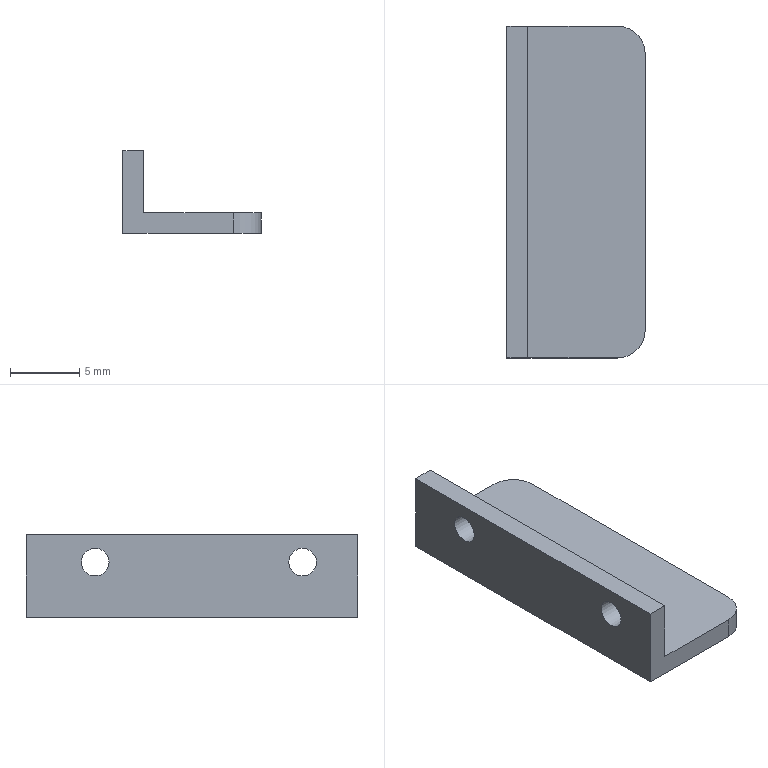Part | STEP file | 1-47.3 | 1 solid | 12 faces | box 10 x 24 x 6 mm | volume 510 mm3 | plane 8 | cylinder 4 | commonest cylinder face diameters 2 x2 4 x2
STEP:
#1=CARTESIAN_POINT('',(0.,0.,0.));
#2=DIRECTION('',(0.,0.,1.));
#3=DIRECTION('',(1.,0.,0.));
#4=AXIS2_PLACEMENT_3D('',#1,#2,#3);
#5=CARTESIAN_POINT('',(-1.5,-12.,-3.));
#6=VERTEX_POINT('',#5);
#7=CARTESIAN_POINT('',(-1.5,12.,-3.));
#8=VERTEX_POINT('',#7);
#9=CARTESIAN_POINT('',(-1.5,-12.,-3.));
#10=DIRECTION('',(0.,1.,0.));
#11=VECTOR('',#10,1.);
#12=LINE('',#9,#11);
#13=CARTESIAN_POINT('',(-1.5,0.,9.));
#14=DIRECTION('',(1.,0.,0.));
#15=DIRECTION('',(0.,1.,0.));
#16=AXIS2_PLACEMENT_3D('',#13,#14,#15);
#17=PLANE('',#16);
#18=CARTESIAN_POINT('',(-12.,-12.));
#19=DIRECTION('',(1.,0.));
#20=VECTOR('',#19,1.);
#21=LINE('',#18,#20);
#22=(GEOMETRIC_REPRESENTATION_CONTEXT(2)PARAMETRIC_REPRESENTATION_CONTEXT()REPRESENTATION_CONTEXT('',''));
#23=DEFINITIONAL_REPRESENTATION('',(#21),#22);
#24=PCURVE('',#17,#23);
#25=CARTESIAN_POINT('',(11.85,0.,-3.));
#26=DIRECTION('',(0.,0.,1.));
#27=DIRECTION('',(0.,1.,0.));
#28=AXIS2_PLACEMENT_3D('',#25,#26,#27);
#29=PLANE('',#28);
#30=CARTESIAN_POINT('',(-12.,13.35));
#31=DIRECTION('',(1.,0.));
#32=VECTOR('',#31,1.);
#33=LINE('',#30,#32);
#34=(GEOMETRIC_REPRESENTATION_CONTEXT(2)PARAMETRIC_REPRESENTATION_CONTEXT()REPRESENTATION_CONTEXT('',''));
#35=DEFINITIONAL_REPRESENTATION('',(#33),#34);
#36=PCURVE('',#29,#35);
#37=SURFACE_CURVE('',#12,(#24,#36),.PCURVE_S1.);
#38=EDGE_CURVE('',#6,#8,#37,.T.);
#39=ORIENTED_EDGE('',*,*,#38,.T.);
#40=CARTESIAN_POINT('',(-1.5,12.,3.));
#41=VERTEX_POINT('',#40);
#42=CARTESIAN_POINT('',(-1.5,12.,-3.));
#43=DIRECTION('',(0.,0.,1.));
#44=VECTOR('',#43,1.);
#45=LINE('',#42,#44);
#46=CARTESIAN_POINT('',(12.,-12.));
#47=DIRECTION('',(0.,1.));
#48=VECTOR('',#47,1.);
#49=LINE('',#46,#48);
#50=(GEOMETRIC_REPRESENTATION_CONTEXT(2)PARAMETRIC_REPRESENTATION_CONTEXT()REPRESENTATION_CONTEXT('',''));
#51=DEFINITIONAL_REPRESENTATION('',(#49),#50);
#52=PCURVE('',#17,#51);
#53=CARTESIAN_POINT('',(3.5,12.,0.));
#54=DIRECTION('',(0.,-1.,0.));
#55=DIRECTION('',(0.,0.,1.));
#56=AXIS2_PLACEMENT_3D('',#53,#54,#55);
#57=PLANE('',#56);
#58=CARTESIAN_POINT('',(-3.,5.));
#59=DIRECTION('',(1.,0.));
#60=VECTOR('',#59,1.);
#61=LINE('',#58,#60);
#62=(GEOMETRIC_REPRESENTATION_CONTEXT(2)PARAMETRIC_REPRESENTATION_CONTEXT()REPRESENTATION_CONTEXT('',''));
#63=DEFINITIONAL_REPRESENTATION('',(#61),#62);
#64=PCURVE('',#57,#63);
#65=SURFACE_CURVE('',#45,(#52,#64),.PCURVE_S1.);
#66=EDGE_CURVE('',#8,#41,#65,.T.);
#67=ORIENTED_EDGE('',*,*,#66,.T.);
#68=CARTESIAN_POINT('',(-1.5,-12.,3.));
#69=VERTEX_POINT('',#68);
#70=CARTESIAN_POINT('',(-1.5,12.,3.));
#71=DIRECTION('',(0.,-1.,0.));
#72=VECTOR('',#71,1.);
#73=LINE('',#70,#72);
#74=CARTESIAN_POINT('',(12.,-6.));
#75=DIRECTION('',(-1.,0.));
#76=VECTOR('',#75,1.);
#77=LINE('',#74,#76);
#78=(GEOMETRIC_REPRESENTATION_CONTEXT(2)PARAMETRIC_REPRESENTATION_CONTEXT()REPRESENTATION_CONTEXT('',''));
#79=DEFINITIONAL_REPRESENTATION('',(#77),#78);
#80=PCURVE('',#17,#79);
#81=CARTESIAN_POINT('',(-0.75,0.,3.));
#82=DIRECTION('',(0.,0.,-1.));
#83=DIRECTION('',(0.,-1.,0.));
#84=AXIS2_PLACEMENT_3D('',#81,#82,#83);
#85=PLANE('',#84);
#86=CARTESIAN_POINT('',(-12.,0.75));
#87=DIRECTION('',(1.,0.));
#88=VECTOR('',#87,1.);
#89=LINE('',#86,#88);
#90=(GEOMETRIC_REPRESENTATION_CONTEXT(2)PARAMETRIC_REPRESENTATION_CONTEXT()REPRESENTATION_CONTEXT('',''));
#91=DEFINITIONAL_REPRESENTATION('',(#89),#90);
#92=PCURVE('',#85,#91);
#93=SURFACE_CURVE('',#73,(#80,#92),.PCURVE_S1.);
#94=EDGE_CURVE('',#41,#69,#93,.T.);
#95=ORIENTED_EDGE('',*,*,#94,.T.);
#96=CARTESIAN_POINT('',(-1.5,-12.,3.));
#97=DIRECTION('',(0.,0.,-1.));
#98=VECTOR('',#97,1.);
#99=LINE('',#96,#98);
#100=CARTESIAN_POINT('',(-12.,-6.));
#101=DIRECTION('',(0.,-1.));
#102=VECTOR('',#101,1.);
#103=LINE('',#100,#102);
#104=(GEOMETRIC_REPRESENTATION_CONTEXT(2)PARAMETRIC_REPRESENTATION_CONTEXT()REPRESENTATION_CONTEXT('',''));
#105=DEFINITIONAL_REPRESENTATION('',(#103),#104);
#106=PCURVE('',#17,#105);
#107=CARTESIAN_POINT('',(3.5,-12.,0.));
#108=DIRECTION('',(0.,1.,0.));
#109=DIRECTION('',(0.,0.,-1.));
#110=AXIS2_PLACEMENT_3D('',#107,#108,#109);
#111=PLANE('',#110);
#112=CARTESIAN_POINT('',(-3.,5.));
#113=DIRECTION('',(1.,0.));
#114=VECTOR('',#113,1.);
#115=LINE('',#112,#114);
#116=(GEOMETRIC_REPRESENTATION_CONTEXT(2)PARAMETRIC_REPRESENTATION_CONTEXT()REPRESENTATION_CONTEXT('',''));
#117=DEFINITIONAL_REPRESENTATION('',(#115),#116);
#118=PCURVE('',#111,#117);
#119=SURFACE_CURVE('',#99,(#106,#118),.PCURVE_S1.);
#120=EDGE_CURVE('',#69,#6,#119,.T.);
#121=ORIENTED_EDGE('',*,*,#120,.T.);
#122=EDGE_LOOP('',(#39,#67,#95,#121));
#123=FACE_BOUND('',#122,.F.);
#124=CARTESIAN_POINT('',(-1.5,-7.,1.));
#125=VERTEX_POINT('',#124);
#126=CARTESIAN_POINT('',(-1.5,-8.,1.));
#127=DIRECTION('',(-1.,0.,0.));
#128=DIRECTION('',(0.,1.,0.));
#129=AXIS2_PLACEMENT_3D('',#126,#127,#128);
#130=CIRCLE('',#129,1.);
#131=CARTESIAN_POINT('',(-7.,-8.));
#132=CARTESIAN_POINT('',(-7.,-9.732));
#133=CARTESIAN_POINT('',(-8.5,-8.866));
#134=CARTESIAN_POINT('',(-10.,-8.));
#135=CARTESIAN_POINT('',(-8.5,-7.134));
#136=CARTESIAN_POINT('',(-7.,-6.268));
#137=CARTESIAN_POINT('',(-7.,-8.));
#138=(BOUNDED_CURVE()B_SPLINE_CURVE(2,(#131,#132,#133,#134,#135,#136,#137),.UNSPECIFIED.,.T.,.F.)B_SPLINE_CURVE_WITH_KNOTS((1,2,2,2,2,1),(-2.094,0.,2.094,4.189,6.283,8.378),.UNSPECIFIED.)CURVE()GEOMETRIC_REPRESENTATION_ITEM()RATIONAL_B_SPLINE_CURVE((1.,0.5,1.,0.5,1.,0.5,1.))REPRESENTATION_ITEM(''));
#139=(GEOMETRIC_REPRESENTATION_CONTEXT(2)PARAMETRIC_REPRESENTATION_CONTEXT()REPRESENTATION_CONTEXT('',''));
#140=DEFINITIONAL_REPRESENTATION('',(#138),#139);
#141=PCURVE('',#17,#140);
#142=CARTESIAN_POINT('',(0.,-8.,1.));
#143=DIRECTION('',(-1.,0.,0.));
#144=DIRECTION('',(0.,1.,0.));
#145=AXIS2_PLACEMENT_3D('',#142,#143,#144);
#146=CYLINDRICAL_SURFACE('',#145,1.);
#147=CARTESIAN_POINT('',(0.,1.5));
#148=DIRECTION('',(1.,0.));
#149=VECTOR('',#148,1.);
#150=LINE('',#147,#149);
#151=(GEOMETRIC_REPRESENTATION_CONTEXT(2)PARAMETRIC_REPRESENTATION_CONTEXT()REPRESENTATION_CONTEXT('',''));
#152=DEFINITIONAL_REPRESENTATION('',(#150),#151);
#153=PCURVE('',#146,#152);
#154=SURFACE_CURVE('',#130,(#141,#153),.PCURVE_S1.);
#155=EDGE_CURVE('',#125,#125,#154,.T.);
#156=ORIENTED_EDGE('',*,*,#155,.T.);
#157=EDGE_LOOP('',(#156));
#158=FACE_BOUND('',#157,.F.);
#159=CARTESIAN_POINT('',(-1.5,8.,1.));
#160=VERTEX_POINT('',#159);
#161=CARTESIAN_POINT('',(-1.5,7.,1.));
#162=DIRECTION('',(-1.,0.,0.));
#163=DIRECTION('',(0.,1.,0.));
#164=AXIS2_PLACEMENT_3D('',#161,#162,#163);
#165=CIRCLE('',#164,1.);
#166=CARTESIAN_POINT('',(8.,-8.));
#167=CARTESIAN_POINT('',(8.,-9.732));
#168=CARTESIAN_POINT('',(6.5,-8.866));
#169=CARTESIAN_POINT('',(5.,-8.));
#170=CARTESIAN_POINT('',(6.5,-7.134));
#171=CARTESIAN_POINT('',(8.,-6.268));
#172=CARTESIAN_POINT('',(8.,-8.));
#173=(BOUNDED_CURVE()B_SPLINE_CURVE(2,(#166,#167,#168,#169,#170,#171,#172),.UNSPECIFIED.,.T.,.F.)B_SPLINE_CURVE_WITH_KNOTS((1,2,2,2,2,1),(-2.094,0.,2.094,4.189,6.283,8.378),.UNSPECIFIED.)CURVE()GEOMETRIC_REPRESENTATION_ITEM()RATIONAL_B_SPLINE_CURVE((1.,0.5,1.,0.5,1.,0.5,1.))REPRESENTATION_ITEM(''));
#174=(GEOMETRIC_REPRESENTATION_CONTEXT(2)PARAMETRIC_REPRESENTATION_CONTEXT()REPRESENTATION_CONTEXT('',''));
#175=DEFINITIONAL_REPRESENTATION('',(#173),#174);
#176=PCURVE('',#17,#175);
#177=CARTESIAN_POINT('',(0.,7.,1.));
#178=DIRECTION('',(-1.,0.,0.));
#179=DIRECTION('',(0.,1.,0.));
#180=AXIS2_PLACEMENT_3D('',#177,#178,#179);
#181=CYLINDRICAL_SURFACE('',#180,1.);
#182=CARTESIAN_POINT('',(0.,1.5));
#183=DIRECTION('',(1.,0.));
#184=VECTOR('',#183,1.);
#185=LINE('',#182,#184);
#186=(GEOMETRIC_REPRESENTATION_CONTEXT(2)PARAMETRIC_REPRESENTATION_CONTEXT()REPRESENTATION_CONTEXT('',''));
#187=DEFINITIONAL_REPRESENTATION('',(#185),#186);
#188=PCURVE('',#181,#187);
#189=SURFACE_CURVE('',#165,(#176,#188),.PCURVE_S1.);
#190=EDGE_CURVE('',#160,#160,#189,.T.);
#191=ORIENTED_EDGE('',*,*,#190,.T.);
#192=EDGE_LOOP('',(#191));
#193=FACE_BOUND('',#192,.F.);
#194=ADVANCED_FACE('',(#123,#158,#193),#17,.F.);
#195=CARTESIAN_POINT('',(0.,12.,3.));
#196=VERTEX_POINT('',#195);
#197=CARTESIAN_POINT('',(0.,-12.,3.));
#198=VERTEX_POINT('',#197);
#199=CARTESIAN_POINT('',(0.,12.,3.));
#200=DIRECTION('',(0.,-1.,0.));
#201=VECTOR('',#200,1.);
#202=LINE('',#199,#201);
#203=CARTESIAN_POINT('',(-12.,-0.75));
#204=DIRECTION('',(1.,0.));
#205=VECTOR('',#204,1.);
#206=LINE('',#203,#205);
#207=(GEOMETRIC_REPRESENTATION_CONTEXT(2)PARAMETRIC_REPRESENTATION_CONTEXT()REPRESENTATION_CONTEXT('',''));
#208=DEFINITIONAL_REPRESENTATION('',(#206),#207);
#209=PCURVE('',#85,#208);
#210=CARTESIAN_POINT('',(0.,0.,9.));
#211=DIRECTION('',(1.,0.,0.));
#212=DIRECTION('',(0.,1.,0.));
#213=AXIS2_PLACEMENT_3D('',#210,#211,#212);
#214=PLANE('',#213);
#215=CARTESIAN_POINT('',(12.,-6.));
#216=DIRECTION('',(-1.,0.));
#217=VECTOR('',#216,1.);
#218=LINE('',#215,#217);
#219=(GEOMETRIC_REPRESENTATION_CONTEXT(2)PARAMETRIC_REPRESENTATION_CONTEXT()REPRESENTATION_CONTEXT('',''));
#220=DEFINITIONAL_REPRESENTATION('',(#218),#219);
#221=PCURVE('',#214,#220);
#222=SURFACE_CURVE('',#202,(#209,#221),.PCURVE_S1.);
#223=EDGE_CURVE('',#196,#198,#222,.T.);
#224=ORIENTED_EDGE('',*,*,#223,.T.);
#225=CARTESIAN_POINT('',(0.,-12.,3.));
#226=DIRECTION('',(-1.,0.,0.));
#227=VECTOR('',#226,1.);
#228=LINE('',#225,#227);
#229=CARTESIAN_POINT('',(12.,-0.75));
#230=DIRECTION('',(0.,1.));
#231=VECTOR('',#230,1.);
#232=LINE('',#229,#231);
#233=(GEOMETRIC_REPRESENTATION_CONTEXT(2)PARAMETRIC_REPRESENTATION_CONTEXT()REPRESENTATION_CONTEXT('',''));
#234=DEFINITIONAL_REPRESENTATION('',(#232),#233);
#235=PCURVE('',#85,#234);
#236=CARTESIAN_POINT('',(-3.,3.5));
#237=DIRECTION('',(0.,1.));
#238=VECTOR('',#237,1.);
#239=LINE('',#236,#238);
#240=(GEOMETRIC_REPRESENTATION_CONTEXT(2)PARAMETRIC_REPRESENTATION_CONTEXT()REPRESENTATION_CONTEXT('',''));
#241=DEFINITIONAL_REPRESENTATION('',(#239),#240);
#242=PCURVE('',#111,#241);
#243=SURFACE_CURVE('',#228,(#235,#242),.PCURVE_S1.);
#244=EDGE_CURVE('',#198,#69,#243,.T.);
#245=ORIENTED_EDGE('',*,*,#244,.T.);
#246=ORIENTED_EDGE('',*,*,#94,.F.);
#247=CARTESIAN_POINT('',(0.,12.,3.));
#248=DIRECTION('',(-1.,0.,0.));
#249=VECTOR('',#248,1.);
#250=LINE('',#247,#249);
#251=CARTESIAN_POINT('',(-12.,-0.75));
#252=DIRECTION('',(0.,1.));
#253=VECTOR('',#252,1.);
#254=LINE('',#251,#253);
#255=(GEOMETRIC_REPRESENTATION_CONTEXT(2)PARAMETRIC_REPRESENTATION_CONTEXT()REPRESENTATION_CONTEXT('',''));
#256=DEFINITIONAL_REPRESENTATION('',(#254),#255);
#257=PCURVE('',#85,#256);
#258=CARTESIAN_POINT('',(3.,3.5));
#259=DIRECTION('',(0.,1.));
#260=VECTOR('',#259,1.);
#261=LINE('',#258,#260);
#262=(GEOMETRIC_REPRESENTATION_CONTEXT(2)PARAMETRIC_REPRESENTATION_CONTEXT()REPRESENTATION_CONTEXT('',''));
#263=DEFINITIONAL_REPRESENTATION('',(#261),#262);
#264=PCURVE('',#57,#263);
#265=SURFACE_CURVE('',#250,(#257,#264),.PCURVE_S1.);
#266=EDGE_CURVE('',#196,#41,#265,.T.);
#267=ORIENTED_EDGE('',*,*,#266,.F.);
#268=EDGE_LOOP('',(#224,#245,#246,#267));
#269=FACE_BOUND('',#268,.F.);
#270=ADVANCED_FACE('',(#269),#85,.F.);
#271=CARTESIAN_POINT('',(0.,-7.,1.));
#272=VERTEX_POINT('',#271);
#273=CARTESIAN_POINT('',(0.,-8.,1.));
#274=DIRECTION('',(-1.,0.,0.));
#275=DIRECTION('',(0.,1.,0.));
#276=AXIS2_PLACEMENT_3D('',#273,#274,#275);
#277=CIRCLE('',#276,1.);
#278=CARTESIAN_POINT('',(0.,0.));
#279=DIRECTION('',(1.,0.));
#280=VECTOR('',#279,1.);
#281=LINE('',#278,#280);
#282=(GEOMETRIC_REPRESENTATION_CONTEXT(2)PARAMETRIC_REPRESENTATION_CONTEXT()REPRESENTATION_CONTEXT('',''));
#283=DEFINITIONAL_REPRESENTATION('',(#281),#282);
#284=PCURVE('',#146,#283);
#285=CARTESIAN_POINT('',(-7.,-8.));
#286=CARTESIAN_POINT('',(-7.,-9.732));
#287=CARTESIAN_POINT('',(-8.5,-8.866));
#288=CARTESIAN_POINT('',(-10.,-8.));
#289=CARTESIAN_POINT('',(-8.5,-7.134));
#290=CARTESIAN_POINT('',(-7.,-6.268));
#291=CARTESIAN_POINT('',(-7.,-8.));
#292=(BOUNDED_CURVE()B_SPLINE_CURVE(2,(#285,#286,#287,#288,#289,#290,#291),.UNSPECIFIED.,.T.,.F.)B_SPLINE_CURVE_WITH_KNOTS((1,2,2,2,2,1),(-2.094,0.,2.094,4.189,6.283,8.378),.UNSPECIFIED.)CURVE()GEOMETRIC_REPRESENTATION_ITEM()RATIONAL_B_SPLINE_CURVE((1.,0.5,1.,0.5,1.,0.5,1.))REPRESENTATION_ITEM(''));
#293=(GEOMETRIC_REPRESENTATION_CONTEXT(2)PARAMETRIC_REPRESENTATION_CONTEXT()REPRESENTATION_CONTEXT('',''));
#294=DEFINITIONAL_REPRESENTATION('',(#292),#293);
#295=PCURVE('',#214,#294);
#296=SURFACE_CURVE('',#277,(#284,#295),.PCURVE_S1.);
#297=EDGE_CURVE('',#272,#272,#296,.T.);
#298=ORIENTED_EDGE('',*,*,#297,.T.);
#299=CARTESIAN_POINT('',(0.,-7.,1.));
#300=DIRECTION('',(-1.,0.,0.));
#301=VECTOR('',#300,1.);
#302=LINE('',#299,#301);
#303=CARTESIAN_POINT('',(6.283,0.));
#304=DIRECTION('',(0.,1.));
#305=VECTOR('',#304,1.);
#306=LINE('',#303,#305);
#307=(GEOMETRIC_REPRESENTATION_CONTEXT(2)PARAMETRIC_REPRESENTATION_CONTEXT()REPRESENTATION_CONTEXT('',''));
#308=DEFINITIONAL_REPRESENTATION('',(#306),#307);
#309=PCURVE('',#146,#308);
#310=CARTESIAN_POINT('',(0.,0.));
#311=DIRECTION('',(0.,1.));
#312=VECTOR('',#311,1.);
#313=LINE('',#310,#312);
#314=(GEOMETRIC_REPRESENTATION_CONTEXT(2)PARAMETRIC_REPRESENTATION_CONTEXT()REPRESENTATION_CONTEXT('',''));
#315=DEFINITIONAL_REPRESENTATION('',(#313),#314);
#316=PCURVE('',#146,#315);
#317=SEAM_CURVE('',#302,(#309,#316),.PCURVE_S1.);
#318=EDGE_CURVE('',#272,#125,#317,.T.);
#319=ORIENTED_EDGE('',*,*,#318,.T.);
#320=ORIENTED_EDGE('',*,*,#155,.F.);
#321=ORIENTED_EDGE('',*,*,#318,.F.);
#322=EDGE_LOOP('',(#298,#319,#320,#321));
#323=FACE_BOUND('',#322,.F.);
#324=ADVANCED_FACE('',(#323),#146,.F.);
#325=CARTESIAN_POINT('',(0.,8.,1.));
#326=VERTEX_POINT('',#325);
#327=CARTESIAN_POINT('',(0.,7.,1.));
#328=DIRECTION('',(-1.,0.,0.));
#329=DIRECTION('',(0.,1.,0.));
#330=AXIS2_PLACEMENT_3D('',#327,#328,#329);
#331=CIRCLE('',#330,1.);
#332=CARTESIAN_POINT('',(0.,0.));
#333=DIRECTION('',(1.,0.));
#334=VECTOR('',#333,1.);
#335=LINE('',#332,#334);
#336=(GEOMETRIC_REPRESENTATION_CONTEXT(2)PARAMETRIC_REPRESENTATION_CONTEXT()REPRESENTATION_CONTEXT('',''));
#337=DEFINITIONAL_REPRESENTATION('',(#335),#336);
#338=PCURVE('',#181,#337);
#339=CARTESIAN_POINT('',(8.,-8.));
#340=CARTESIAN_POINT('',(8.,-9.732));
#341=CARTESIAN_POINT('',(6.5,-8.866));
#342=CARTESIAN_POINT('',(5.,-8.));
#343=CARTESIAN_POINT('',(6.5,-7.134));
#344=CARTESIAN_POINT('',(8.,-6.268));
#345=CARTESIAN_POINT('',(8.,-8.));
#346=(BOUNDED_CURVE()B_SPLINE_CURVE(2,(#339,#340,#341,#342,#343,#344,#345),.UNSPECIFIED.,.T.,.F.)B_SPLINE_CURVE_WITH_KNOTS((1,2,2,2,2,1),(-2.094,0.,2.094,4.189,6.283,8.378),.UNSPECIFIED.)CURVE()GEOMETRIC_REPRESENTATION_ITEM()RATIONAL_B_SPLINE_CURVE((1.,0.5,1.,0.5,1.,0.5,1.))REPRESENTATION_ITEM(''));
#347=(GEOMETRIC_REPRESENTATION_CONTEXT(2)PARAMETRIC_REPRESENTATION_CONTEXT()REPRESENTATION_CONTEXT('',''));
#348=DEFINITIONAL_REPRESENTATION('',(#346),#347);
#349=PCURVE('',#214,#348);
#350=SURFACE_CURVE('',#331,(#338,#349),.PCURVE_S1.);
#351=EDGE_CURVE('',#326,#326,#350,.T.);
#352=ORIENTED_EDGE('',*,*,#351,.T.);
#353=CARTESIAN_POINT('',(0.,8.,1.));
#354=DIRECTION('',(-1.,0.,0.));
#355=VECTOR('',#354,1.);
#356=LINE('',#353,#355);
#357=CARTESIAN_POINT('',(6.283,0.));
#358=DIRECTION('',(0.,1.));
#359=VECTOR('',#358,1.);
#360=LINE('',#357,#359);
#361=(GEOMETRIC_REPRESENTATION_CONTEXT(2)PARAMETRIC_REPRESENTATION_CONTEXT()REPRESENTATION_CONTEXT('',''));
#362=DEFINITIONAL_REPRESENTATION('',(#360),#361);
#363=PCURVE('',#181,#362);
#364=CARTESIAN_POINT('',(0.,0.));
#365=DIRECTION('',(0.,1.));
#366=VECTOR('',#365,1.);
#367=LINE('',#364,#366);
#368=(GEOMETRIC_REPRESENTATION_CONTEXT(2)PARAMETRIC_REPRESENTATION_CONTEXT()REPRESENTATION_CONTEXT('',''));
#369=DEFINITIONAL_REPRESENTATION('',(#367),#368);
#370=PCURVE('',#181,#369);
#371=SEAM_CURVE('',#356,(#363,#370),.PCURVE_S1.);
#372=EDGE_CURVE('',#326,#160,#371,.T.);
#373=ORIENTED_EDGE('',*,*,#372,.T.);
#374=ORIENTED_EDGE('',*,*,#190,.F.);
#375=ORIENTED_EDGE('',*,*,#372,.F.);
#376=EDGE_LOOP('',(#352,#373,#374,#375));
#377=FACE_BOUND('',#376,.F.);
#378=ADVANCED_FACE('',(#377),#181,.F.);
#379=ORIENTED_EDGE('',*,*,#223,.T.);
#380=CARTESIAN_POINT('',(0.,-12.,-1.5));
#381=VERTEX_POINT('',#380);
#382=CARTESIAN_POINT('',(0.,-12.,3.));
#383=DIRECTION('',(0.,0.,-1.));
#384=VECTOR('',#383,1.);
#385=LINE('',#382,#384);
#386=CARTESIAN_POINT('',(-12.,-6.));
#387=DIRECTION('',(0.,-1.));
#388=VECTOR('',#387,1.);
#389=LINE('',#386,#388);
#390=(GEOMETRIC_REPRESENTATION_CONTEXT(2)PARAMETRIC_REPRESENTATION_CONTEXT()REPRESENTATION_CONTEXT('',''));
#391=DEFINITIONAL_REPRESENTATION('',(#389),#390);
#392=PCURVE('',#214,#391);
#393=CARTESIAN_POINT('',(-3.,3.5));
#394=DIRECTION('',(1.,0.));
#395=VECTOR('',#394,1.);
#396=LINE('',#393,#395);
#397=(GEOMETRIC_REPRESENTATION_CONTEXT(2)PARAMETRIC_REPRESENTATION_CONTEXT()REPRESENTATION_CONTEXT('',''));
#398=DEFINITIONAL_REPRESENTATION('',(#396),#397);
#399=PCURVE('',#111,#398);
#400=SURFACE_CURVE('',#385,(#392,#399),.PCURVE_S1.);
#401=EDGE_CURVE('',#198,#381,#400,.T.);
#402=ORIENTED_EDGE('',*,*,#401,.T.);
#403=CARTESIAN_POINT('',(0.,12.,-1.5));
#404=VERTEX_POINT('',#403);
#405=CARTESIAN_POINT('',(0.,-12.,-1.5));
#406=DIRECTION('',(0.,1.,0.));
#407=VECTOR('',#406,1.);
#408=LINE('',#405,#407);
#409=CARTESIAN_POINT('',(-12.,-10.5));
#410=DIRECTION('',(1.,0.));
#411=VECTOR('',#410,1.);
#412=LINE('',#409,#411);
#413=(GEOMETRIC_REPRESENTATION_CONTEXT(2)PARAMETRIC_REPRESENTATION_CONTEXT()REPRESENTATION_CONTEXT('',''));
#414=DEFINITIONAL_REPRESENTATION('',(#412),#413);
#415=PCURVE('',#214,#414);
#416=CARTESIAN_POINT('',(12.,-1.682,-1.5));
#417=DIRECTION('',(0.,0.,-1.));
#418=DIRECTION('',(0.,1.,0.));
#419=AXIS2_PLACEMENT_3D('',#416,#417,#418);
#420=PLANE('',#419);
#421=CARTESIAN_POINT('',(-10.318,-12.));
#422=DIRECTION('',(1.,0.));
#423=VECTOR('',#422,1.);
#424=LINE('',#421,#423);
#425=(GEOMETRIC_REPRESENTATION_CONTEXT(2)PARAMETRIC_REPRESENTATION_CONTEXT()REPRESENTATION_CONTEXT('',''));
#426=DEFINITIONAL_REPRESENTATION('',(#424),#425);
#427=PCURVE('',#420,#426);
#428=SURFACE_CURVE('',#408,(#415,#427),.PCURVE_S1.);
#429=EDGE_CURVE('',#381,#404,#428,.T.);
#430=ORIENTED_EDGE('',*,*,#429,.T.);
#431=CARTESIAN_POINT('',(0.,12.,-1.5));
#432=DIRECTION('',(0.,0.,1.));
#433=VECTOR('',#432,1.);
#434=LINE('',#431,#433);
#435=CARTESIAN_POINT('',(12.,-10.5));
#436=DIRECTION('',(0.,1.));
#437=VECTOR('',#436,1.);
#438=LINE('',#435,#437);
#439=(GEOMETRIC_REPRESENTATION_CONTEXT(2)PARAMETRIC_REPRESENTATION_CONTEXT()REPRESENTATION_CONTEXT('',''));
#440=DEFINITIONAL_REPRESENTATION('',(#438),#439);
#441=PCURVE('',#214,#440);
#442=CARTESIAN_POINT('',(-1.5,3.5));
#443=DIRECTION('',(1.,0.));
#444=VECTOR('',#443,1.);
#445=LINE('',#442,#444);
#446=(GEOMETRIC_REPRESENTATION_CONTEXT(2)PARAMETRIC_REPRESENTATION_CONTEXT()REPRESENTATION_CONTEXT('',''));
#447=DEFINITIONAL_REPRESENTATION('',(#445),#446);
#448=PCURVE('',#57,#447);
#449=SURFACE_CURVE('',#434,(#441,#448),.PCURVE_S1.);
#450=EDGE_CURVE('',#404,#196,#449,.T.);
#451=ORIENTED_EDGE('',*,*,#450,.T.);
#452=EDGE_LOOP('',(#379,#402,#430,#451));
#453=FACE_BOUND('',#452,.T.);
#454=ORIENTED_EDGE('',*,*,#297,.T.);
#455=EDGE_LOOP('',(#454));
#456=FACE_BOUND('',#455,.T.);
#457=ORIENTED_EDGE('',*,*,#351,.T.);
#458=EDGE_LOOP('',(#457));
#459=FACE_BOUND('',#458,.T.);
#460=ADVANCED_FACE('',(#453,#456,#459),#214,.T.);
#461=ORIENTED_EDGE('',*,*,#38,.F.);
#462=CARTESIAN_POINT('',(6.5,-12.,-3.));
#463=VERTEX_POINT('',#462);
#464=CARTESIAN_POINT('',(-1.5,-12.,-3.));
#465=DIRECTION('',(1.,0.,0.));
#466=VECTOR('',#465,1.);
#467=LINE('',#464,#466);
#468=CARTESIAN_POINT('',(-12.,13.35));
#469=DIRECTION('',(0.,-1.));
#470=VECTOR('',#469,1.);
#471=LINE('',#468,#470);
#472=(GEOMETRIC_REPRESENTATION_CONTEXT(2)PARAMETRIC_REPRESENTATION_CONTEXT()REPRESENTATION_CONTEXT('',''));
#473=DEFINITIONAL_REPRESENTATION('',(#471),#472);
#474=PCURVE('',#29,#473);
#475=CARTESIAN_POINT('',(3.,5.));
#476=DIRECTION('',(0.,-1.));
#477=VECTOR('',#476,1.);
#478=LINE('',#475,#477);
#479=(GEOMETRIC_REPRESENTATION_CONTEXT(2)PARAMETRIC_REPRESENTATION_CONTEXT()REPRESENTATION_CONTEXT('',''));
#480=DEFINITIONAL_REPRESENTATION('',(#478),#479);
#481=PCURVE('',#111,#480);
#482=SURFACE_CURVE('',#467,(#474,#481),.PCURVE_S1.);
#483=EDGE_CURVE('',#6,#463,#482,.T.);
#484=ORIENTED_EDGE('',*,*,#483,.T.);
#485=CARTESIAN_POINT('',(8.5,-10.,-3.));
#486=VERTEX_POINT('',#485);
#487=CARTESIAN_POINT('',(6.5,-10.,-3.));
#488=DIRECTION('',(0.,0.,-1.));
#489=DIRECTION('',(1.,0.,0.));
#490=AXIS2_PLACEMENT_3D('',#487,#488,#489);
#491=CIRCLE('',#490,2.);
#492=CARTESIAN_POINT('',(-10.,3.35));
#493=CARTESIAN_POINT('',(-13.464,3.35));
#494=CARTESIAN_POINT('',(-11.732,6.35));
#495=CARTESIAN_POINT('',(-10.,9.35));
#496=CARTESIAN_POINT('',(-8.268,6.35));
#497=CARTESIAN_POINT('',(-6.536,3.35));
#498=CARTESIAN_POINT('',(-10.,3.35));
#499=(BOUNDED_CURVE()B_SPLINE_CURVE(2,(#492,#493,#494,#495,#496,#497,#498),.UNSPECIFIED.,.T.,.F.)B_SPLINE_CURVE_WITH_KNOTS((1,2,2,2,2,1),(-2.094,0.,2.094,4.189,6.283,8.378),.UNSPECIFIED.)CURVE()GEOMETRIC_REPRESENTATION_ITEM()RATIONAL_B_SPLINE_CURVE((1.,0.5,1.,0.5,1.,0.5,1.))REPRESENTATION_ITEM(''));
#500=(GEOMETRIC_REPRESENTATION_CONTEXT(2)PARAMETRIC_REPRESENTATION_CONTEXT()REPRESENTATION_CONTEXT('',''));
#501=DEFINITIONAL_REPRESENTATION('',(#499),#500);
#502=PCURVE('',#29,#501);
#503=CARTESIAN_POINT('',(6.5,-10.,-3.));
#504=DIRECTION('',(0.,0.,1.));
#505=DIRECTION('',(1.,0.,0.));
#506=AXIS2_PLACEMENT_3D('',#503,#504,#505);
#507=CYLINDRICAL_SURFACE('',#506,2.);
#508=CARTESIAN_POINT('',(6.283,0.));
#509=DIRECTION('',(-1.,0.));
#510=VECTOR('',#509,1.);
#511=LINE('',#508,#510);
#512=(GEOMETRIC_REPRESENTATION_CONTEXT(2)PARAMETRIC_REPRESENTATION_CONTEXT()REPRESENTATION_CONTEXT('',''));
#513=DEFINITIONAL_REPRESENTATION('',(#511),#512);
#514=PCURVE('',#507,#513);
#515=SURFACE_CURVE('',#491,(#502,#514),.PCURVE_S1.);
#516=EDGE_CURVE('',#486,#463,#515,.T.);
#517=ORIENTED_EDGE('',*,*,#516,.F.);
#518=CARTESIAN_POINT('',(8.5,10.,-3.));
#519=VERTEX_POINT('',#518);
#520=CARTESIAN_POINT('',(8.5,10.,-3.));
#521=DIRECTION('',(0.,-1.,0.));
#522=VECTOR('',#521,1.);
#523=LINE('',#520,#522);
#524=CARTESIAN_POINT('',(10.,3.35));
#525=DIRECTION('',(-1.,0.));
#526=VECTOR('',#525,1.);
#527=LINE('',#524,#526);
#528=(GEOMETRIC_REPRESENTATION_CONTEXT(2)PARAMETRIC_REPRESENTATION_CONTEXT()REPRESENTATION_CONTEXT('',''));
#529=DEFINITIONAL_REPRESENTATION('',(#527),#528);
#530=PCURVE('',#29,#529);
#531=CARTESIAN_POINT('',(8.5,0.,0.));
#532=DIRECTION('',(-1.,0.,0.));
#533=DIRECTION('',(0.,-1.,0.));
#534=AXIS2_PLACEMENT_3D('',#531,#532,#533);
#535=PLANE('',#534);
#536=CARTESIAN_POINT('',(-10.,-3.));
#537=DIRECTION('',(1.,0.));
#538=VECTOR('',#537,1.);
#539=LINE('',#536,#538);
#540=(GEOMETRIC_REPRESENTATION_CONTEXT(2)PARAMETRIC_REPRESENTATION_CONTEXT()REPRESENTATION_CONTEXT('',''));
#541=DEFINITIONAL_REPRESENTATION('',(#539),#540);
#542=PCURVE('',#535,#541);
#543=SURFACE_CURVE('',#523,(#530,#542),.PCURVE_S1.);
#544=EDGE_CURVE('',#519,#486,#543,.T.);
#545=ORIENTED_EDGE('',*,*,#544,.F.);
#546=CARTESIAN_POINT('',(6.5,12.,-3.));
#547=VERTEX_POINT('',#546);
#548=CARTESIAN_POINT('',(6.5,10.,-3.));
#549=DIRECTION('',(0.,0.,-1.));
#550=DIRECTION('',(0.,1.,0.));
#551=AXIS2_PLACEMENT_3D('',#548,#549,#550);
#552=CIRCLE('',#551,2.);
#553=CARTESIAN_POINT('',(12.,5.35));
#554=CARTESIAN_POINT('',(12.,1.886));
#555=CARTESIAN_POINT('',(9.,3.618));
#556=CARTESIAN_POINT('',(6.,5.35));
#557=CARTESIAN_POINT('',(9.,7.082));
#558=CARTESIAN_POINT('',(12.,8.814));
#559=CARTESIAN_POINT('',(12.,5.35));
#560=(BOUNDED_CURVE()B_SPLINE_CURVE(2,(#553,#554,#555,#556,#557,#558,#559),.UNSPECIFIED.,.T.,.F.)B_SPLINE_CURVE_WITH_KNOTS((1,2,2,2,2,1),(-2.094,0.,2.094,4.189,6.283,8.378),.UNSPECIFIED.)CURVE()GEOMETRIC_REPRESENTATION_ITEM()RATIONAL_B_SPLINE_CURVE((1.,0.5,1.,0.5,1.,0.5,1.))REPRESENTATION_ITEM(''));
#561=(GEOMETRIC_REPRESENTATION_CONTEXT(2)PARAMETRIC_REPRESENTATION_CONTEXT()REPRESENTATION_CONTEXT('',''));
#562=DEFINITIONAL_REPRESENTATION('',(#560),#561);
#563=PCURVE('',#29,#562);
#564=CARTESIAN_POINT('',(6.5,10.,-3.));
#565=DIRECTION('',(0.,0.,1.));
#566=DIRECTION('',(0.,1.,0.));
#567=AXIS2_PLACEMENT_3D('',#564,#565,#566);
#568=CYLINDRICAL_SURFACE('',#567,2.);
#569=CARTESIAN_POINT('',(6.283,0.));
#570=DIRECTION('',(-1.,0.));
#571=VECTOR('',#570,1.);
#572=LINE('',#569,#571);
#573=(GEOMETRIC_REPRESENTATION_CONTEXT(2)PARAMETRIC_REPRESENTATION_CONTEXT()REPRESENTATION_CONTEXT('',''));
#574=DEFINITIONAL_REPRESENTATION('',(#572),#573);
#575=PCURVE('',#568,#574);
#576=SURFACE_CURVE('',#552,(#563,#575),.PCURVE_S1.);
#577=EDGE_CURVE('',#547,#519,#576,.T.);
#578=ORIENTED_EDGE('',*,*,#577,.F.);
#579=CARTESIAN_POINT('',(6.5,12.,-3.));
#580=DIRECTION('',(-1.,0.,0.));
#581=VECTOR('',#580,1.);
#582=LINE('',#579,#581);
#583=CARTESIAN_POINT('',(12.,5.35));
#584=DIRECTION('',(0.,1.));
#585=VECTOR('',#584,1.);
#586=LINE('',#583,#585);
#587=(GEOMETRIC_REPRESENTATION_CONTEXT(2)PARAMETRIC_REPRESENTATION_CONTEXT()REPRESENTATION_CONTEXT('',''));
#588=DEFINITIONAL_REPRESENTATION('',(#586),#587);
#589=PCURVE('',#29,#588);
#590=CARTESIAN_POINT('',(-3.,-3.));
#591=DIRECTION('',(0.,1.));
#592=VECTOR('',#591,1.);
#593=LINE('',#590,#592);
#594=(GEOMETRIC_REPRESENTATION_CONTEXT(2)PARAMETRIC_REPRESENTATION_CONTEXT()REPRESENTATION_CONTEXT('',''));
#595=DEFINITIONAL_REPRESENTATION('',(#593),#594);
#596=PCURVE('',#57,#595);
#597=SURFACE_CURVE('',#582,(#589,#596),.PCURVE_S1.);
#598=EDGE_CURVE('',#547,#8,#597,.T.);
#599=ORIENTED_EDGE('',*,*,#598,.T.);
#600=EDGE_LOOP('',(#461,#484,#517,#545,#578,#599));
#601=FACE_BOUND('',#600,.F.);
#602=ADVANCED_FACE('',(#601),#29,.F.);
#603=ORIENTED_EDGE('',*,*,#450,.T.);
#604=ORIENTED_EDGE('',*,*,#266,.T.);
#605=ORIENTED_EDGE('',*,*,#66,.F.);
#606=ORIENTED_EDGE('',*,*,#598,.F.);
#607=CARTESIAN_POINT('',(6.5,12.,-1.5));
#608=VERTEX_POINT('',#607);
#609=CARTESIAN_POINT('',(6.5,12.,-3.));
#610=DIRECTION('',(0.,0.,1.));
#611=VECTOR('',#610,1.);
#612=LINE('',#609,#611);
#613=CARTESIAN_POINT('',(-3.,-3.));
#614=DIRECTION('',(1.,0.));
#615=VECTOR('',#614,1.);
#616=LINE('',#613,#615);
#617=(GEOMETRIC_REPRESENTATION_CONTEXT(2)PARAMETRIC_REPRESENTATION_CONTEXT()REPRESENTATION_CONTEXT('',''));
#618=DEFINITIONAL_REPRESENTATION('',(#616),#617);
#619=PCURVE('',#57,#618);
#620=CARTESIAN_POINT('',(6.283,0.));
#621=DIRECTION('',(0.,1.));
#622=VECTOR('',#621,1.);
#623=LINE('',#620,#622);
#624=(GEOMETRIC_REPRESENTATION_CONTEXT(2)PARAMETRIC_REPRESENTATION_CONTEXT()REPRESENTATION_CONTEXT('',''));
#625=DEFINITIONAL_REPRESENTATION('',(#623),#624);
#626=PCURVE('',#568,#625);
#627=SURFACE_CURVE('',#612,(#619,#626),.PCURVE_S1.);
#628=EDGE_CURVE('',#547,#608,#627,.T.);
#629=ORIENTED_EDGE('',*,*,#628,.T.);
#630=CARTESIAN_POINT('',(0.,12.,-1.5));
#631=DIRECTION('',(1.,0.,0.));
#632=VECTOR('',#631,1.);
#633=LINE('',#630,#632);
#634=CARTESIAN_POINT('',(-1.5,3.5));
#635=DIRECTION('',(0.,-1.));
#636=VECTOR('',#635,1.);
#637=LINE('',#634,#636);
#638=(GEOMETRIC_REPRESENTATION_CONTEXT(2)PARAMETRIC_REPRESENTATION_CONTEXT()REPRESENTATION_CONTEXT('',''));
#639=DEFINITIONAL_REPRESENTATION('',(#637),#638);
#640=PCURVE('',#57,#639);
#641=CARTESIAN_POINT('',(13.682,-12.));
#642=DIRECTION('',(0.,1.));
#643=VECTOR('',#642,1.);
#644=LINE('',#641,#643);
#645=(GEOMETRIC_REPRESENTATION_CONTEXT(2)PARAMETRIC_REPRESENTATION_CONTEXT()REPRESENTATION_CONTEXT('',''));
#646=DEFINITIONAL_REPRESENTATION('',(#644),#645);
#647=PCURVE('',#420,#646);
#648=SURFACE_CURVE('',#633,(#640,#647),.PCURVE_S1.);
#649=EDGE_CURVE('',#404,#608,#648,.T.);
#650=ORIENTED_EDGE('',*,*,#649,.F.);
#651=EDGE_LOOP('',(#603,#604,#605,#606,#629,#650));
#652=FACE_BOUND('',#651,.F.);
#653=ADVANCED_FACE('',(#652),#57,.F.);
#654=ORIENTED_EDGE('',*,*,#120,.F.);
#655=ORIENTED_EDGE('',*,*,#244,.F.);
#656=ORIENTED_EDGE('',*,*,#401,.T.);
#657=CARTESIAN_POINT('',(6.5,-12.,-1.5));
#658=VERTEX_POINT('',#657);
#659=CARTESIAN_POINT('',(6.5,-12.,-1.5));
#660=DIRECTION('',(-1.,0.,0.));
#661=VECTOR('',#660,1.);
#662=LINE('',#659,#661);
#663=CARTESIAN_POINT('',(1.5,-3.));
#664=DIRECTION('',(0.,1.));
#665=VECTOR('',#664,1.);
#666=LINE('',#663,#665);
#667=(GEOMETRIC_REPRESENTATION_CONTEXT(2)PARAMETRIC_REPRESENTATION_CONTEXT()REPRESENTATION_CONTEXT('',''));
#668=DEFINITIONAL_REPRESENTATION('',(#666),#667);
#669=PCURVE('',#111,#668);
#670=CARTESIAN_POINT('',(-10.318,-5.5));
#671=DIRECTION('',(0.,-1.));
#672=VECTOR('',#671,1.);
#673=LINE('',#670,#672);
#674=(GEOMETRIC_REPRESENTATION_CONTEXT(2)PARAMETRIC_REPRESENTATION_CONTEXT()REPRESENTATION_CONTEXT('',''));
#675=DEFINITIONAL_REPRESENTATION('',(#673),#674);
#676=PCURVE('',#420,#675);
#677=SURFACE_CURVE('',#662,(#669,#676),.PCURVE_S1.);
#678=EDGE_CURVE('',#658,#381,#677,.T.);
#679=ORIENTED_EDGE('',*,*,#678,.F.);
#680=CARTESIAN_POINT('',(6.5,-12.,-3.));
#681=DIRECTION('',(0.,0.,1.));
#682=VECTOR('',#681,1.);
#683=LINE('',#680,#682);
#684=CARTESIAN_POINT('',(3.,-3.));
#685=DIRECTION('',(-1.,0.));
#686=VECTOR('',#685,1.);
#687=LINE('',#684,#686);
#688=(GEOMETRIC_REPRESENTATION_CONTEXT(2)PARAMETRIC_REPRESENTATION_CONTEXT()REPRESENTATION_CONTEXT('',''));
#689=DEFINITIONAL_REPRESENTATION('',(#687),#688);
#690=PCURVE('',#111,#689);
#691=CARTESIAN_POINT('',(4.712,0.));
#692=DIRECTION('',(0.,1.));
#693=VECTOR('',#692,1.);
#694=LINE('',#691,#693);
#695=(GEOMETRIC_REPRESENTATION_CONTEXT(2)PARAMETRIC_REPRESENTATION_CONTEXT()REPRESENTATION_CONTEXT('',''));
#696=DEFINITIONAL_REPRESENTATION('',(#694),#695);
#697=PCURVE('',#507,#696);
#698=SURFACE_CURVE('',#683,(#690,#697),.PCURVE_S1.);
#699=EDGE_CURVE('',#463,#658,#698,.T.);
#700=ORIENTED_EDGE('',*,*,#699,.F.);
#701=ORIENTED_EDGE('',*,*,#483,.F.);
#702=EDGE_LOOP('',(#654,#655,#656,#679,#700,#701));
#703=FACE_BOUND('',#702,.F.);
#704=ADVANCED_FACE('',(#703),#111,.F.);
#705=ORIENTED_EDGE('',*,*,#544,.T.);
#706=CARTESIAN_POINT('',(8.5,-10.,-1.5));
#707=VERTEX_POINT('',#706);
#708=CARTESIAN_POINT('',(8.5,-10.,-3.));
#709=DIRECTION('',(0.,0.,1.));
#710=VECTOR('',#709,1.);
#711=LINE('',#708,#710);
#712=CARTESIAN_POINT('',(10.,-3.));
#713=DIRECTION('',(0.,1.));
#714=VECTOR('',#713,1.);
#715=LINE('',#712,#714);
#716=(GEOMETRIC_REPRESENTATION_CONTEXT(2)PARAMETRIC_REPRESENTATION_CONTEXT()REPRESENTATION_CONTEXT('',''));
#717=DEFINITIONAL_REPRESENTATION('',(#715),#716);
#718=PCURVE('',#535,#717);
#719=CARTESIAN_POINT('',(6.283,0.));
#720=DIRECTION('',(0.,1.));
#721=VECTOR('',#720,1.);
#722=LINE('',#719,#721);
#723=(GEOMETRIC_REPRESENTATION_CONTEXT(2)PARAMETRIC_REPRESENTATION_CONTEXT()REPRESENTATION_CONTEXT('',''));
#724=DEFINITIONAL_REPRESENTATION('',(#722),#723);
#725=PCURVE('',#507,#724);
#726=SURFACE_CURVE('',#711,(#718,#725),.PCURVE_S1.);
#727=EDGE_CURVE('',#486,#707,#726,.T.);
#728=ORIENTED_EDGE('',*,*,#727,.T.);
#729=CARTESIAN_POINT('',(8.5,10.,-1.5));
#730=VERTEX_POINT('',#729);
#731=CARTESIAN_POINT('',(8.5,10.,-1.5));
#732=DIRECTION('',(0.,-1.,0.));
#733=VECTOR('',#732,1.);
#734=LINE('',#731,#733);
#735=CARTESIAN_POINT('',(-10.,-1.5));
#736=DIRECTION('',(1.,0.));
#737=VECTOR('',#736,1.);
#738=LINE('',#735,#737);
#739=(GEOMETRIC_REPRESENTATION_CONTEXT(2)PARAMETRIC_REPRESENTATION_CONTEXT()REPRESENTATION_CONTEXT('',''));
#740=DEFINITIONAL_REPRESENTATION('',(#738),#739);
#741=PCURVE('',#535,#740);
#742=CARTESIAN_POINT('',(11.682,-3.5));
#743=DIRECTION('',(-1.,0.));
#744=VECTOR('',#743,1.);
#745=LINE('',#742,#744);
#746=(GEOMETRIC_REPRESENTATION_CONTEXT(2)PARAMETRIC_REPRESENTATION_CONTEXT()REPRESENTATION_CONTEXT('',''));
#747=DEFINITIONAL_REPRESENTATION('',(#745),#746);
#748=PCURVE('',#420,#747);
#749=SURFACE_CURVE('',#734,(#741,#748),.PCURVE_S1.);
#750=EDGE_CURVE('',#730,#707,#749,.T.);
#751=ORIENTED_EDGE('',*,*,#750,.F.);
#752=CARTESIAN_POINT('',(8.5,10.,-3.));
#753=DIRECTION('',(0.,0.,1.));
#754=VECTOR('',#753,1.);
#755=LINE('',#752,#754);
#756=CARTESIAN_POINT('',(-10.,-3.));
#757=DIRECTION('',(0.,1.));
#758=VECTOR('',#757,1.);
#759=LINE('',#756,#758);
#760=(GEOMETRIC_REPRESENTATION_CONTEXT(2)PARAMETRIC_REPRESENTATION_CONTEXT()REPRESENTATION_CONTEXT('',''));
#761=DEFINITIONAL_REPRESENTATION('',(#759),#760);
#762=PCURVE('',#535,#761);
#763=CARTESIAN_POINT('',(4.712,0.));
#764=DIRECTION('',(0.,1.));
#765=VECTOR('',#764,1.);
#766=LINE('',#763,#765);
#767=(GEOMETRIC_REPRESENTATION_CONTEXT(2)PARAMETRIC_REPRESENTATION_CONTEXT()REPRESENTATION_CONTEXT('',''));
#768=DEFINITIONAL_REPRESENTATION('',(#766),#767);
#769=PCURVE('',#568,#768);
#770=SURFACE_CURVE('',#755,(#762,#769),.PCURVE_S1.);
#771=EDGE_CURVE('',#519,#730,#770,.T.);
#772=ORIENTED_EDGE('',*,*,#771,.F.);
#773=EDGE_LOOP('',(#705,#728,#751,#772));
#774=FACE_BOUND('',#773,.F.);
#775=ADVANCED_FACE('',(#774),#535,.F.);
#776=ORIENTED_EDGE('',*,*,#429,.T.);
#777=ORIENTED_EDGE('',*,*,#649,.T.);
#778=CARTESIAN_POINT('',(6.5,10.,-1.5));
#779=DIRECTION('',(0.,0.,1.));
#780=DIRECTION('',(1.,0.,0.));
#781=AXIS2_PLACEMENT_3D('',#778,#779,#780);
#782=CIRCLE('',#781,2.);
#783=CARTESIAN_POINT('',(11.682,-3.5));
#784=CARTESIAN_POINT('',(15.146,-3.5));
#785=CARTESIAN_POINT('',(13.414,-6.5));
#786=CARTESIAN_POINT('',(11.682,-9.5));
#787=CARTESIAN_POINT('',(9.95,-6.5));
#788=CARTESIAN_POINT('',(8.218,-3.5));
#789=CARTESIAN_POINT('',(11.682,-3.5));
#790=(BOUNDED_CURVE()B_SPLINE_CURVE(2,(#783,#784,#785,#786,#787,#788,#789),.UNSPECIFIED.,.T.,.F.)B_SPLINE_CURVE_WITH_KNOTS((1,2,2,2,2,1),(-2.094,0.,2.094,4.189,6.283,8.378),.UNSPECIFIED.)CURVE()GEOMETRIC_REPRESENTATION_ITEM()RATIONAL_B_SPLINE_CURVE((1.,0.5,1.,0.5,1.,0.5,1.))REPRESENTATION_ITEM(''));
#791=(GEOMETRIC_REPRESENTATION_CONTEXT(2)PARAMETRIC_REPRESENTATION_CONTEXT()REPRESENTATION_CONTEXT('',''));
#792=DEFINITIONAL_REPRESENTATION('',(#790),#791);
#793=PCURVE('',#420,#792);
#794=CARTESIAN_POINT('',(4.712,1.5));
#795=DIRECTION('',(1.,0.));
#796=VECTOR('',#795,1.);
#797=LINE('',#794,#796);
#798=(GEOMETRIC_REPRESENTATION_CONTEXT(2)PARAMETRIC_REPRESENTATION_CONTEXT()REPRESENTATION_CONTEXT('',''));
#799=DEFINITIONAL_REPRESENTATION('',(#797),#798);
#800=PCURVE('',#568,#799);
#801=SURFACE_CURVE('',#782,(#793,#800),.PCURVE_S1.);
#802=EDGE_CURVE('',#730,#608,#801,.T.);
#803=ORIENTED_EDGE('',*,*,#802,.F.);
#804=ORIENTED_EDGE('',*,*,#750,.T.);
#805=CARTESIAN_POINT('',(6.5,-10.,-1.5));
#806=DIRECTION('',(0.,0.,1.));
#807=DIRECTION('',(0.,-1.,0.));
#808=AXIS2_PLACEMENT_3D('',#805,#806,#807);
#809=CIRCLE('',#808,2.);
#810=CARTESIAN_POINT('',(-10.318,-5.5));
#811=CARTESIAN_POINT('',(-10.318,-2.036));
#812=CARTESIAN_POINT('',(-7.318,-3.768));
#813=CARTESIAN_POINT('',(-4.318,-5.5));
#814=CARTESIAN_POINT('',(-7.318,-7.232));
#815=CARTESIAN_POINT('',(-10.318,-8.964));
#816=CARTESIAN_POINT('',(-10.318,-5.5));
#817=(BOUNDED_CURVE()B_SPLINE_CURVE(2,(#810,#811,#812,#813,#814,#815,#816),.UNSPECIFIED.,.T.,.F.)B_SPLINE_CURVE_WITH_KNOTS((1,2,2,2,2,1),(-2.094,0.,2.094,4.189,6.283,8.378),.UNSPECIFIED.)CURVE()GEOMETRIC_REPRESENTATION_ITEM()RATIONAL_B_SPLINE_CURVE((1.,0.5,1.,0.5,1.,0.5,1.))REPRESENTATION_ITEM(''));
#818=(GEOMETRIC_REPRESENTATION_CONTEXT(2)PARAMETRIC_REPRESENTATION_CONTEXT()REPRESENTATION_CONTEXT('',''));
#819=DEFINITIONAL_REPRESENTATION('',(#817),#818);
#820=PCURVE('',#420,#819);
#821=CARTESIAN_POINT('',(4.712,1.5));
#822=DIRECTION('',(1.,0.));
#823=VECTOR('',#822,1.);
#824=LINE('',#821,#823);
#825=(GEOMETRIC_REPRESENTATION_CONTEXT(2)PARAMETRIC_REPRESENTATION_CONTEXT()REPRESENTATION_CONTEXT('',''));
#826=DEFINITIONAL_REPRESENTATION('',(#824),#825);
#827=PCURVE('',#507,#826);
#828=SURFACE_CURVE('',#809,(#820,#827),.PCURVE_S1.);
#829=EDGE_CURVE('',#658,#707,#828,.T.);
#830=ORIENTED_EDGE('',*,*,#829,.F.);
#831=ORIENTED_EDGE('',*,*,#678,.T.);
#832=EDGE_LOOP('',(#776,#777,#803,#804,#830,#831));
#833=FACE_BOUND('',#832,.F.);
#834=ADVANCED_FACE('',(#833),#420,.F.);
#835=ORIENTED_EDGE('',*,*,#727,.T.);
#836=ORIENTED_EDGE('',*,*,#829,.F.);
#837=ORIENTED_EDGE('',*,*,#699,.F.);
#838=ORIENTED_EDGE('',*,*,#516,.F.);
#839=EDGE_LOOP('',(#835,#836,#837,#838));
#840=FACE_BOUND('',#839,.T.);
#841=ADVANCED_FACE('',(#840),#507,.T.);
#842=ORIENTED_EDGE('',*,*,#628,.T.);
#843=ORIENTED_EDGE('',*,*,#802,.F.);
#844=ORIENTED_EDGE('',*,*,#771,.F.);
#845=ORIENTED_EDGE('',*,*,#577,.F.);
#846=EDGE_LOOP('',(#842,#843,#844,#845));
#847=FACE_BOUND('',#846,.T.);
#848=ADVANCED_FACE('',(#847),#568,.T.);
#849=CLOSED_SHELL('',(#194,#270,#324,#378,#460,#602,#653,#704,#775,#834,#841,#848));
#850=MANIFOLD_SOLID_BREP('',#849);
#851=(LENGTH_UNIT()NAMED_UNIT(*)SI_UNIT(.MILLI.,.METRE.));
#852=UNCERTAINTY_MEASURE_WITH_UNIT(LENGTH_MEASURE(0.0000001),#851,'','');
#853=(NAMED_UNIT(*)PLANE_ANGLE_UNIT()SI_UNIT($,.RADIAN.));
#854=(NAMED_UNIT(*)SI_UNIT($,.STERADIAN.)SOLID_ANGLE_UNIT());
#855=(GEOMETRIC_REPRESENTATION_CONTEXT(3)GLOBAL_UNCERTAINTY_ASSIGNED_CONTEXT((#852))GLOBAL_UNIT_ASSIGNED_CONTEXT((#851,#853,#854))REPRESENTATION_CONTEXT('',''));
#856=ADVANCED_BREP_SHAPE_REPRESENTATION('',(#4,#850),#855);